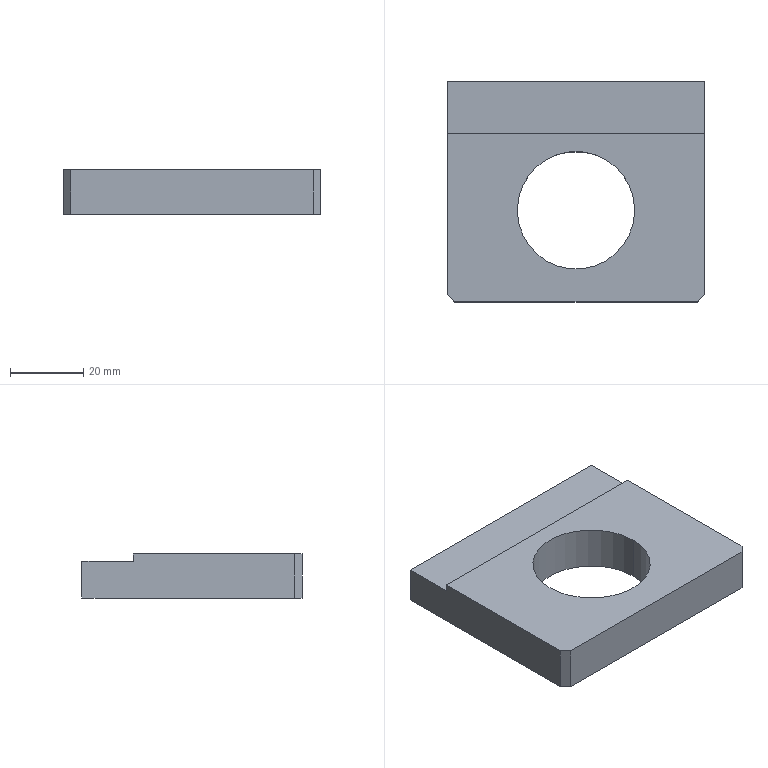Part | STEP file | 2012-06-08-07 | 1 solid | 12 faces | box 70 x 60 x 12 mm | volume 38741 mm3 | plane 10 | cylinder 2 | commonest cylinder face diameters 32 x2
STEP:
#1=CARTESIAN_POINT('',(0.,0.,0.));
#2=DIRECTION('',(0.,0.,1.));
#3=DIRECTION('',(1.,0.,0.));
#4=AXIS2_PLACEMENT_3D('',#1,#2,#3);
#5=CARTESIAN_POINT('',(-16.,-5.,12.));
#6=VERTEX_POINT('',#5);
#7=CARTESIAN_POINT('',(-16.,-5.,0.));
#8=VERTEX_POINT('',#7);
#9=CARTESIAN_POINT('',(-16.,-5.,12.));
#10=DIRECTION('',(0.,0.,-1.));
#11=VECTOR('',#10,1.);
#12=LINE('',#9,#11);
#13=CARTESIAN_POINT('',(0.,-5.,12.));
#14=DIRECTION('',(0.,0.,-1.));
#15=DIRECTION('',(-1.,0.,0.));
#16=AXIS2_PLACEMENT_3D('',#13,#14,#15);
#17=CYLINDRICAL_SURFACE('',#16,16.);
#18=CARTESIAN_POINT('',(6.283,0.));
#19=DIRECTION('',(0.,1.));
#20=VECTOR('',#19,1.);
#21=LINE('',#18,#20);
#22=(GEOMETRIC_REPRESENTATION_CONTEXT(2)PARAMETRIC_REPRESENTATION_CONTEXT()REPRESENTATION_CONTEXT('',''));
#23=DEFINITIONAL_REPRESENTATION('',(#21),#22);
#24=PCURVE('',#17,#23);
#25=CARTESIAN_POINT('',(0.,-5.,12.));
#26=DIRECTION('',(0.,0.,-1.));
#27=DIRECTION('',(-1.,0.,0.));
#28=AXIS2_PLACEMENT_3D('',#25,#26,#27);
#29=CYLINDRICAL_SURFACE('',#28,16.);
#30=CARTESIAN_POINT('',(0.,0.));
#31=DIRECTION('',(0.,1.));
#32=VECTOR('',#31,1.);
#33=LINE('',#30,#32);
#34=(GEOMETRIC_REPRESENTATION_CONTEXT(2)PARAMETRIC_REPRESENTATION_CONTEXT()REPRESENTATION_CONTEXT('',''));
#35=DEFINITIONAL_REPRESENTATION('',(#33),#34);
#36=PCURVE('',#29,#35);
#37=SURFACE_CURVE('',#12,(#24,#36),.PCURVE_S1.);
#38=EDGE_CURVE('',#6,#8,#37,.T.);
#39=ORIENTED_EDGE('',*,*,#38,.T.);
#40=CARTESIAN_POINT('',(16.,-5.,0.));
#41=VERTEX_POINT('',#40);
#42=CARTESIAN_POINT('',(0.,-5.,0.));
#43=DIRECTION('',(0.,0.,1.));
#44=DIRECTION('',(1.,0.,0.));
#45=AXIS2_PLACEMENT_3D('',#42,#43,#44);
#46=CIRCLE('',#45,16.);
#47=CARTESIAN_POINT('',(9.425,12.));
#48=DIRECTION('',(-1.,0.));
#49=VECTOR('',#48,1.);
#50=LINE('',#47,#49);
#51=(GEOMETRIC_REPRESENTATION_CONTEXT(2)PARAMETRIC_REPRESENTATION_CONTEXT()REPRESENTATION_CONTEXT('',''));
#52=DEFINITIONAL_REPRESENTATION('',(#50),#51);
#53=PCURVE('',#17,#52);
#54=CARTESIAN_POINT('',(35.,-30.,0.));
#55=DIRECTION('',(0.,0.,1.));
#56=DIRECTION('',(1.,0.,0.));
#57=AXIS2_PLACEMENT_3D('',#54,#55,#56);
#58=PLANE('',#57);
#59=CARTESIAN_POINT('',(-35.,25.));
#60=DIRECTION('',(1.,0.));
#61=AXIS2_PLACEMENT_2D('',#59,#60);
#62=CIRCLE('',#61,16.);
#63=(GEOMETRIC_REPRESENTATION_CONTEXT(2)PARAMETRIC_REPRESENTATION_CONTEXT()REPRESENTATION_CONTEXT('',''));
#64=DEFINITIONAL_REPRESENTATION('',(#62),#63);
#65=PCURVE('',#58,#64);
#66=SURFACE_CURVE('',#46,(#53,#65),.PCURVE_S1.);
#67=EDGE_CURVE('',#8,#41,#66,.T.);
#68=ORIENTED_EDGE('',*,*,#67,.T.);
#69=CARTESIAN_POINT('',(16.,-5.,12.));
#70=VERTEX_POINT('',#69);
#71=CARTESIAN_POINT('',(16.,-5.,12.));
#72=DIRECTION('',(0.,0.,-1.));
#73=VECTOR('',#72,1.);
#74=LINE('',#71,#73);
#75=CARTESIAN_POINT('',(3.142,0.));
#76=DIRECTION('',(0.,1.));
#77=VECTOR('',#76,1.);
#78=LINE('',#75,#77);
#79=(GEOMETRIC_REPRESENTATION_CONTEXT(2)PARAMETRIC_REPRESENTATION_CONTEXT()REPRESENTATION_CONTEXT('',''));
#80=DEFINITIONAL_REPRESENTATION('',(#78),#79);
#81=PCURVE('',#17,#80);
#82=CARTESIAN_POINT('',(3.142,0.));
#83=DIRECTION('',(0.,1.));
#84=VECTOR('',#83,1.);
#85=LINE('',#82,#84);
#86=(GEOMETRIC_REPRESENTATION_CONTEXT(2)PARAMETRIC_REPRESENTATION_CONTEXT()REPRESENTATION_CONTEXT('',''));
#87=DEFINITIONAL_REPRESENTATION('',(#85),#86);
#88=PCURVE('',#29,#87);
#89=SURFACE_CURVE('',#74,(#81,#88),.PCURVE_S1.);
#90=EDGE_CURVE('',#70,#41,#89,.T.);
#91=ORIENTED_EDGE('',*,*,#90,.F.);
#92=CARTESIAN_POINT('',(0.,-5.,12.));
#93=DIRECTION('',(0.,0.,1.));
#94=DIRECTION('',(1.,0.,0.));
#95=AXIS2_PLACEMENT_3D('',#92,#93,#94);
#96=CIRCLE('',#95,16.);
#97=CARTESIAN_POINT('',(9.425,0.));
#98=DIRECTION('',(-1.,0.));
#99=VECTOR('',#98,1.);
#100=LINE('',#97,#99);
#101=(GEOMETRIC_REPRESENTATION_CONTEXT(2)PARAMETRIC_REPRESENTATION_CONTEXT()REPRESENTATION_CONTEXT('',''));
#102=DEFINITIONAL_REPRESENTATION('',(#100),#101);
#103=PCURVE('',#17,#102);
#104=CARTESIAN_POINT('',(35.,-30.,12.));
#105=DIRECTION('',(0.,0.,1.));
#106=DIRECTION('',(1.,0.,0.));
#107=AXIS2_PLACEMENT_3D('',#104,#105,#106);
#108=PLANE('',#107);
#109=CARTESIAN_POINT('',(-35.,25.));
#110=DIRECTION('',(1.,0.));
#111=AXIS2_PLACEMENT_2D('',#109,#110);
#112=CIRCLE('',#111,16.);
#113=(GEOMETRIC_REPRESENTATION_CONTEXT(2)PARAMETRIC_REPRESENTATION_CONTEXT()REPRESENTATION_CONTEXT('',''));
#114=DEFINITIONAL_REPRESENTATION('',(#112),#113);
#115=PCURVE('',#108,#114);
#116=SURFACE_CURVE('',#96,(#103,#115),.PCURVE_S1.);
#117=EDGE_CURVE('',#6,#70,#116,.T.);
#118=ORIENTED_EDGE('',*,*,#117,.F.);
#119=EDGE_LOOP('',(#39,#68,#91,#118));
#120=FACE_BOUND('',#119,.F.);
#121=ADVANCED_FACE('',(#120),#17,.F.);
#122=CARTESIAN_POINT('',(35.,30.,10.));
#123=VERTEX_POINT('',#122);
#124=CARTESIAN_POINT('',(-35.,30.,10.));
#125=VERTEX_POINT('',#124);
#126=CARTESIAN_POINT('',(-35.,30.,10.));
#127=DIRECTION('',(-1.,0.,0.));
#128=VECTOR('',#127,1.);
#129=LINE('',#126,#128);
#130=CARTESIAN_POINT('',(-35.,30.,12.));
#131=DIRECTION('',(0.,-1.,0.));
#132=DIRECTION('',(0.,0.,-1.));
#133=AXIS2_PLACEMENT_3D('',#130,#131,#132);
#134=PLANE('',#133);
#135=CARTESIAN_POINT('',(2.,0.));
#136=DIRECTION('',(0.,-1.));
#137=VECTOR('',#136,1.);
#138=LINE('',#135,#137);
#139=(GEOMETRIC_REPRESENTATION_CONTEXT(2)PARAMETRIC_REPRESENTATION_CONTEXT()REPRESENTATION_CONTEXT('',''));
#140=DEFINITIONAL_REPRESENTATION('',(#138),#139);
#141=PCURVE('',#134,#140);
#142=CARTESIAN_POINT('',(-35.,16.,10.));
#143=DIRECTION('',(0.,0.,1.));
#144=DIRECTION('',(1.,0.,0.));
#145=AXIS2_PLACEMENT_3D('',#142,#143,#144);
#146=PLANE('',#145);
#147=CARTESIAN_POINT('',(0.,14.));
#148=DIRECTION('',(-1.,0.));
#149=VECTOR('',#148,1.);
#150=LINE('',#147,#149);
#151=(GEOMETRIC_REPRESENTATION_CONTEXT(2)PARAMETRIC_REPRESENTATION_CONTEXT()REPRESENTATION_CONTEXT('',''));
#152=DEFINITIONAL_REPRESENTATION('',(#150),#151);
#153=PCURVE('',#146,#152);
#154=SURFACE_CURVE('',#129,(#141,#153),.PCURVE_S1.);
#155=EDGE_CURVE('',#123,#125,#154,.T.);
#156=ORIENTED_EDGE('',*,*,#155,.F.);
#157=CARTESIAN_POINT('',(35.,30.,0.));
#158=VERTEX_POINT('',#157);
#159=CARTESIAN_POINT('',(35.,30.,12.));
#160=DIRECTION('',(0.,0.,-1.));
#161=VECTOR('',#160,1.);
#162=LINE('',#159,#161);
#163=CARTESIAN_POINT('',(0.,70.));
#164=DIRECTION('',(1.,0.));
#165=VECTOR('',#164,1.);
#166=LINE('',#163,#165);
#167=(GEOMETRIC_REPRESENTATION_CONTEXT(2)PARAMETRIC_REPRESENTATION_CONTEXT()REPRESENTATION_CONTEXT('',''));
#168=DEFINITIONAL_REPRESENTATION('',(#166),#167);
#169=PCURVE('',#134,#168);
#170=CARTESIAN_POINT('',(35.,30.,12.));
#171=DIRECTION('',(-1.,0.,0.));
#172=DIRECTION('',(0.,0.,1.));
#173=AXIS2_PLACEMENT_3D('',#170,#171,#172);
#174=PLANE('',#173);
#175=CARTESIAN_POINT('',(0.,0.));
#176=DIRECTION('',(-1.,0.));
#177=VECTOR('',#176,1.);
#178=LINE('',#175,#177);
#179=(GEOMETRIC_REPRESENTATION_CONTEXT(2)PARAMETRIC_REPRESENTATION_CONTEXT()REPRESENTATION_CONTEXT('',''));
#180=DEFINITIONAL_REPRESENTATION('',(#178),#179);
#181=PCURVE('',#174,#180);
#182=SURFACE_CURVE('',#162,(#169,#181),.PCURVE_S1.);
#183=EDGE_CURVE('',#123,#158,#182,.T.);
#184=ORIENTED_EDGE('',*,*,#183,.T.);
#185=CARTESIAN_POINT('',(-35.,30.,0.));
#186=VERTEX_POINT('',#185);
#187=CARTESIAN_POINT('',(-35.,30.,0.));
#188=DIRECTION('',(-1.,0.,0.));
#189=VECTOR('',#188,1.);
#190=LINE('',#187,#189);
#191=CARTESIAN_POINT('',(12.,0.));
#192=DIRECTION('',(0.,-1.));
#193=VECTOR('',#192,1.);
#194=LINE('',#191,#193);
#195=(GEOMETRIC_REPRESENTATION_CONTEXT(2)PARAMETRIC_REPRESENTATION_CONTEXT()REPRESENTATION_CONTEXT('',''));
#196=DEFINITIONAL_REPRESENTATION('',(#194),#195);
#197=PCURVE('',#134,#196);
#198=CARTESIAN_POINT('',(-70.,60.));
#199=DIRECTION('',(-1.,0.));
#200=VECTOR('',#199,1.);
#201=LINE('',#198,#200);
#202=(GEOMETRIC_REPRESENTATION_CONTEXT(2)PARAMETRIC_REPRESENTATION_CONTEXT()REPRESENTATION_CONTEXT('',''));
#203=DEFINITIONAL_REPRESENTATION('',(#201),#202);
#204=PCURVE('',#58,#203);
#205=SURFACE_CURVE('',#190,(#197,#204),.PCURVE_S1.);
#206=EDGE_CURVE('',#158,#186,#205,.T.);
#207=ORIENTED_EDGE('',*,*,#206,.T.);
#208=CARTESIAN_POINT('',(-35.,30.,12.));
#209=DIRECTION('',(0.,0.,-1.));
#210=VECTOR('',#209,1.);
#211=LINE('',#208,#210);
#212=CARTESIAN_POINT('',(0.,0.));
#213=DIRECTION('',(1.,0.));
#214=VECTOR('',#213,1.);
#215=LINE('',#212,#214);
#216=(GEOMETRIC_REPRESENTATION_CONTEXT(2)PARAMETRIC_REPRESENTATION_CONTEXT()REPRESENTATION_CONTEXT('',''));
#217=DEFINITIONAL_REPRESENTATION('',(#215),#216);
#218=PCURVE('',#134,#217);
#219=CARTESIAN_POINT('',(-35.,30.,12.));
#220=DIRECTION('',(1.,0.,0.));
#221=DIRECTION('',(0.,1.,0.));
#222=AXIS2_PLACEMENT_3D('',#219,#220,#221);
#223=PLANE('',#222);
#224=CARTESIAN_POINT('',(0.,0.));
#225=DIRECTION('',(0.,-1.));
#226=VECTOR('',#225,1.);
#227=LINE('',#224,#226);
#228=(GEOMETRIC_REPRESENTATION_CONTEXT(2)PARAMETRIC_REPRESENTATION_CONTEXT()REPRESENTATION_CONTEXT('',''));
#229=DEFINITIONAL_REPRESENTATION('',(#227),#228);
#230=PCURVE('',#223,#229);
#231=SURFACE_CURVE('',#211,(#218,#230),.PCURVE_S1.);
#232=EDGE_CURVE('',#125,#186,#231,.T.);
#233=ORIENTED_EDGE('',*,*,#232,.F.);
#234=EDGE_LOOP('',(#156,#184,#207,#233));
#235=FACE_BOUND('',#234,.T.);
#236=ADVANCED_FACE('',(#235),#134,.F.);
#237=CARTESIAN_POINT('',(-33.,-30.,12.));
#238=VERTEX_POINT('',#237);
#239=CARTESIAN_POINT('',(33.,-30.,12.));
#240=VERTEX_POINT('',#239);
#241=CARTESIAN_POINT('',(-35.,-30.,12.));
#242=DIRECTION('',(1.,0.,0.));
#243=VECTOR('',#242,1.);
#244=LINE('',#241,#243);
#245=CARTESIAN_POINT('',(-70.,0.));
#246=DIRECTION('',(1.,0.));
#247=VECTOR('',#246,1.);
#248=LINE('',#245,#247);
#249=(GEOMETRIC_REPRESENTATION_CONTEXT(2)PARAMETRIC_REPRESENTATION_CONTEXT()REPRESENTATION_CONTEXT('',''));
#250=DEFINITIONAL_REPRESENTATION('',(#248),#249);
#251=PCURVE('',#108,#250);
#252=CARTESIAN_POINT('',(-35.,-30.,12.));
#253=DIRECTION('',(0.,1.,0.));
#254=DIRECTION('',(0.,0.,1.));
#255=AXIS2_PLACEMENT_3D('',#252,#253,#254);
#256=PLANE('',#255);
#257=CARTESIAN_POINT('',(0.,0.));
#258=DIRECTION('',(0.,1.));
#259=VECTOR('',#258,1.);
#260=LINE('',#257,#259);
#261=(GEOMETRIC_REPRESENTATION_CONTEXT(2)PARAMETRIC_REPRESENTATION_CONTEXT()REPRESENTATION_CONTEXT('',''));
#262=DEFINITIONAL_REPRESENTATION('',(#260),#261);
#263=PCURVE('',#256,#262);
#264=SURFACE_CURVE('',#244,(#251,#263),.PCURVE_S1.);
#265=EDGE_CURVE('',#238,#240,#264,.T.);
#266=ORIENTED_EDGE('',*,*,#265,.T.);
#267=CARTESIAN_POINT('',(35.,-28.,12.));
#268=VERTEX_POINT('',#267);
#269=CARTESIAN_POINT('',(34.,-29.,12.));
#270=DIRECTION('',(0.7071,0.7071,0.));
#271=VECTOR('',#270,1.);
#272=LINE('',#269,#271);
#273=CARTESIAN_POINT('',(-1.,1.));
#274=DIRECTION('',(0.7071,0.7071));
#275=VECTOR('',#274,1.);
#276=LINE('',#273,#275);
#277=(GEOMETRIC_REPRESENTATION_CONTEXT(2)PARAMETRIC_REPRESENTATION_CONTEXT()REPRESENTATION_CONTEXT('',''));
#278=DEFINITIONAL_REPRESENTATION('',(#276),#277);
#279=PCURVE('',#108,#278);
#280=CARTESIAN_POINT('',(35.,-28.,12.));
#281=DIRECTION('',(-0.7071,0.7071,0.));
#282=DIRECTION('',(-0.7071,-0.7071,0.));
#283=AXIS2_PLACEMENT_3D('',#280,#281,#282);
#284=PLANE('',#283);
#285=CARTESIAN_POINT('',(1.414,0.));
#286=DIRECTION('',(-1.,0.));
#287=VECTOR('',#286,1.);
#288=LINE('',#285,#287);
#289=(GEOMETRIC_REPRESENTATION_CONTEXT(2)PARAMETRIC_REPRESENTATION_CONTEXT()REPRESENTATION_CONTEXT('',''));
#290=DEFINITIONAL_REPRESENTATION('',(#288),#289);
#291=PCURVE('',#284,#290);
#292=SURFACE_CURVE('',#272,(#279,#291),.PCURVE_S1.);
#293=EDGE_CURVE('',#240,#268,#292,.T.);
#294=ORIENTED_EDGE('',*,*,#293,.T.);
#295=CARTESIAN_POINT('',(35.,16.,12.));
#296=VERTEX_POINT('',#295);
#297=CARTESIAN_POINT('',(35.,30.,12.));
#298=DIRECTION('',(0.,1.,0.));
#299=VECTOR('',#298,1.);
#300=LINE('',#297,#299);
#301=CARTESIAN_POINT('',(0.,60.));
#302=DIRECTION('',(0.,1.));
#303=VECTOR('',#302,1.);
#304=LINE('',#301,#303);
#305=(GEOMETRIC_REPRESENTATION_CONTEXT(2)PARAMETRIC_REPRESENTATION_CONTEXT()REPRESENTATION_CONTEXT('',''));
#306=DEFINITIONAL_REPRESENTATION('',(#304),#305);
#307=PCURVE('',#108,#306);
#308=CARTESIAN_POINT('',(0.,0.));
#309=DIRECTION('',(0.,1.));
#310=VECTOR('',#309,1.);
#311=LINE('',#308,#310);
#312=(GEOMETRIC_REPRESENTATION_CONTEXT(2)PARAMETRIC_REPRESENTATION_CONTEXT()REPRESENTATION_CONTEXT('',''));
#313=DEFINITIONAL_REPRESENTATION('',(#311),#312);
#314=PCURVE('',#174,#313);
#315=SURFACE_CURVE('',#300,(#307,#314),.PCURVE_S1.);
#316=EDGE_CURVE('',#268,#296,#315,.T.);
#317=ORIENTED_EDGE('',*,*,#316,.T.);
#318=CARTESIAN_POINT('',(-35.,16.,12.));
#319=VERTEX_POINT('',#318);
#320=CARTESIAN_POINT('',(-35.,16.,12.));
#321=DIRECTION('',(1.,0.,0.));
#322=VECTOR('',#321,1.);
#323=LINE('',#320,#322);
#324=CARTESIAN_POINT('',(-70.,46.));
#325=DIRECTION('',(1.,0.));
#326=VECTOR('',#325,1.);
#327=LINE('',#324,#326);
#328=(GEOMETRIC_REPRESENTATION_CONTEXT(2)PARAMETRIC_REPRESENTATION_CONTEXT()REPRESENTATION_CONTEXT('',''));
#329=DEFINITIONAL_REPRESENTATION('',(#327),#328);
#330=PCURVE('',#108,#329);
#331=CARTESIAN_POINT('',(-35.,16.,10.));
#332=DIRECTION('',(0.,-1.,0.));
#333=DIRECTION('',(0.,0.,-1.));
#334=AXIS2_PLACEMENT_3D('',#331,#332,#333);
#335=PLANE('',#334);
#336=CARTESIAN_POINT('',(-2.,0.));
#337=DIRECTION('',(0.,1.));
#338=VECTOR('',#337,1.);
#339=LINE('',#336,#338);
#340=(GEOMETRIC_REPRESENTATION_CONTEXT(2)PARAMETRIC_REPRESENTATION_CONTEXT()REPRESENTATION_CONTEXT('',''));
#341=DEFINITIONAL_REPRESENTATION('',(#339),#340);
#342=PCURVE('',#335,#341);
#343=SURFACE_CURVE('',#323,(#330,#342),.PCURVE_S1.);
#344=EDGE_CURVE('',#319,#296,#343,.T.);
#345=ORIENTED_EDGE('',*,*,#344,.F.);
#346=CARTESIAN_POINT('',(-35.,-28.,12.));
#347=VERTEX_POINT('',#346);
#348=CARTESIAN_POINT('',(-35.,30.,12.));
#349=DIRECTION('',(0.,-1.,0.));
#350=VECTOR('',#349,1.);
#351=LINE('',#348,#350);
#352=CARTESIAN_POINT('',(-70.,60.));
#353=DIRECTION('',(0.,-1.));
#354=VECTOR('',#353,1.);
#355=LINE('',#352,#354);
#356=(GEOMETRIC_REPRESENTATION_CONTEXT(2)PARAMETRIC_REPRESENTATION_CONTEXT()REPRESENTATION_CONTEXT('',''));
#357=DEFINITIONAL_REPRESENTATION('',(#355),#356);
#358=PCURVE('',#108,#357);
#359=CARTESIAN_POINT('',(0.,0.));
#360=DIRECTION('',(-1.,0.));
#361=VECTOR('',#360,1.);
#362=LINE('',#359,#361);
#363=(GEOMETRIC_REPRESENTATION_CONTEXT(2)PARAMETRIC_REPRESENTATION_CONTEXT()REPRESENTATION_CONTEXT('',''));
#364=DEFINITIONAL_REPRESENTATION('',(#362),#363);
#365=PCURVE('',#223,#364);
#366=SURFACE_CURVE('',#351,(#358,#365),.PCURVE_S1.);
#367=EDGE_CURVE('',#319,#347,#366,.T.);
#368=ORIENTED_EDGE('',*,*,#367,.T.);
#369=CARTESIAN_POINT('',(1.,-64.,12.));
#370=DIRECTION('',(0.7071,-0.7071,0.));
#371=VECTOR('',#370,1.);
#372=LINE('',#369,#371);
#373=CARTESIAN_POINT('',(-34.,-34.));
#374=DIRECTION('',(0.7071,-0.7071));
#375=VECTOR('',#374,1.);
#376=LINE('',#373,#375);
#377=(GEOMETRIC_REPRESENTATION_CONTEXT(2)PARAMETRIC_REPRESENTATION_CONTEXT()REPRESENTATION_CONTEXT('',''));
#378=DEFINITIONAL_REPRESENTATION('',(#376),#377);
#379=PCURVE('',#108,#378);
#380=CARTESIAN_POINT('',(-33.,-30.,12.));
#381=DIRECTION('',(0.7071,0.7071,0.));
#382=DIRECTION('',(-0.7071,0.7071,0.));
#383=AXIS2_PLACEMENT_3D('',#380,#381,#382);
#384=PLANE('',#383);
#385=CARTESIAN_POINT('',(-48.083,0.));
#386=DIRECTION('',(-1.,0.));
#387=VECTOR('',#386,1.);
#388=LINE('',#385,#387);
#389=(GEOMETRIC_REPRESENTATION_CONTEXT(2)PARAMETRIC_REPRESENTATION_CONTEXT()REPRESENTATION_CONTEXT('',''));
#390=DEFINITIONAL_REPRESENTATION('',(#388),#389);
#391=PCURVE('',#384,#390);
#392=SURFACE_CURVE('',#372,(#379,#391),.PCURVE_S1.);
#393=EDGE_CURVE('',#347,#238,#392,.T.);
#394=ORIENTED_EDGE('',*,*,#393,.T.);
#395=EDGE_LOOP('',(#266,#294,#317,#345,#368,#394));
#396=FACE_BOUND('',#395,.T.);
#397=ORIENTED_EDGE('',*,*,#117,.F.);
#398=CARTESIAN_POINT('',(0.,-5.,12.));
#399=DIRECTION('',(0.,0.,1.));
#400=DIRECTION('',(1.,0.,0.));
#401=AXIS2_PLACEMENT_3D('',#398,#399,#400);
#402=CIRCLE('',#401,16.);
#403=CARTESIAN_POINT('',(-35.,25.));
#404=DIRECTION('',(1.,0.));
#405=AXIS2_PLACEMENT_2D('',#403,#404);
#406=CIRCLE('',#405,16.);
#407=(GEOMETRIC_REPRESENTATION_CONTEXT(2)PARAMETRIC_REPRESENTATION_CONTEXT()REPRESENTATION_CONTEXT('',''));
#408=DEFINITIONAL_REPRESENTATION('',(#406),#407);
#409=PCURVE('',#108,#408);
#410=CARTESIAN_POINT('',(3.142,0.));
#411=DIRECTION('',(-1.,0.));
#412=VECTOR('',#411,1.);
#413=LINE('',#410,#412);
#414=(GEOMETRIC_REPRESENTATION_CONTEXT(2)PARAMETRIC_REPRESENTATION_CONTEXT()REPRESENTATION_CONTEXT('',''));
#415=DEFINITIONAL_REPRESENTATION('',(#413),#414);
#416=PCURVE('',#29,#415);
#417=SURFACE_CURVE('',#402,(#409,#416),.PCURVE_S1.);
#418=EDGE_CURVE('',#70,#6,#417,.T.);
#419=ORIENTED_EDGE('',*,*,#418,.F.);
#420=EDGE_LOOP('',(#397,#419));
#421=FACE_BOUND('',#420,.T.);
#422=ADVANCED_FACE('',(#396,#421),#108,.T.);
#423=CARTESIAN_POINT('',(35.,-28.,0.));
#424=VERTEX_POINT('',#423);
#425=CARTESIAN_POINT('',(35.,30.,0.));
#426=DIRECTION('',(0.,1.,0.));
#427=VECTOR('',#426,1.);
#428=LINE('',#425,#427);
#429=CARTESIAN_POINT('',(0.,60.));
#430=DIRECTION('',(0.,1.));
#431=VECTOR('',#430,1.);
#432=LINE('',#429,#431);
#433=(GEOMETRIC_REPRESENTATION_CONTEXT(2)PARAMETRIC_REPRESENTATION_CONTEXT()REPRESENTATION_CONTEXT('',''));
#434=DEFINITIONAL_REPRESENTATION('',(#432),#433);
#435=PCURVE('',#58,#434);
#436=CARTESIAN_POINT('',(-12.,0.));
#437=DIRECTION('',(0.,1.));
#438=VECTOR('',#437,1.);
#439=LINE('',#436,#438);
#440=(GEOMETRIC_REPRESENTATION_CONTEXT(2)PARAMETRIC_REPRESENTATION_CONTEXT()REPRESENTATION_CONTEXT('',''));
#441=DEFINITIONAL_REPRESENTATION('',(#439),#440);
#442=PCURVE('',#174,#441);
#443=SURFACE_CURVE('',#428,(#435,#442),.PCURVE_S1.);
#444=EDGE_CURVE('',#424,#158,#443,.T.);
#445=ORIENTED_EDGE('',*,*,#444,.F.);
#446=CARTESIAN_POINT('',(33.,-30.,0.));
#447=VERTEX_POINT('',#446);
#448=CARTESIAN_POINT('',(35.,-28.,0.));
#449=DIRECTION('',(-0.7071,-0.7071,0.));
#450=VECTOR('',#449,1.);
#451=LINE('',#448,#450);
#452=CARTESIAN_POINT('',(0.,2.));
#453=DIRECTION('',(-0.7071,-0.7071));
#454=VECTOR('',#453,1.);
#455=LINE('',#452,#454);
#456=(GEOMETRIC_REPRESENTATION_CONTEXT(2)PARAMETRIC_REPRESENTATION_CONTEXT()REPRESENTATION_CONTEXT('',''));
#457=DEFINITIONAL_REPRESENTATION('',(#455),#456);
#458=PCURVE('',#58,#457);
#459=CARTESIAN_POINT('',(0.,-12.));
#460=DIRECTION('',(1.,0.));
#461=VECTOR('',#460,1.);
#462=LINE('',#459,#461);
#463=(GEOMETRIC_REPRESENTATION_CONTEXT(2)PARAMETRIC_REPRESENTATION_CONTEXT()REPRESENTATION_CONTEXT('',''));
#464=DEFINITIONAL_REPRESENTATION('',(#462),#463);
#465=PCURVE('',#284,#464);
#466=SURFACE_CURVE('',#451,(#458,#465),.PCURVE_S1.);
#467=EDGE_CURVE('',#424,#447,#466,.T.);
#468=ORIENTED_EDGE('',*,*,#467,.T.);
#469=CARTESIAN_POINT('',(-33.,-30.,0.));
#470=VERTEX_POINT('',#469);
#471=CARTESIAN_POINT('',(-35.,-30.,0.));
#472=DIRECTION('',(1.,0.,0.));
#473=VECTOR('',#472,1.);
#474=LINE('',#471,#473);
#475=CARTESIAN_POINT('',(-70.,0.));
#476=DIRECTION('',(1.,0.));
#477=VECTOR('',#476,1.);
#478=LINE('',#475,#477);
#479=(GEOMETRIC_REPRESENTATION_CONTEXT(2)PARAMETRIC_REPRESENTATION_CONTEXT()REPRESENTATION_CONTEXT('',''));
#480=DEFINITIONAL_REPRESENTATION('',(#478),#479);
#481=PCURVE('',#58,#480);
#482=CARTESIAN_POINT('',(-12.,0.));
#483=DIRECTION('',(0.,1.));
#484=VECTOR('',#483,1.);
#485=LINE('',#482,#484);
#486=(GEOMETRIC_REPRESENTATION_CONTEXT(2)PARAMETRIC_REPRESENTATION_CONTEXT()REPRESENTATION_CONTEXT('',''));
#487=DEFINITIONAL_REPRESENTATION('',(#485),#486);
#488=PCURVE('',#256,#487);
#489=SURFACE_CURVE('',#474,(#481,#488),.PCURVE_S1.);
#490=EDGE_CURVE('',#470,#447,#489,.T.);
#491=ORIENTED_EDGE('',*,*,#490,.F.);
#492=CARTESIAN_POINT('',(-35.,-28.,0.));
#493=VERTEX_POINT('',#492);
#494=CARTESIAN_POINT('',(-33.,-30.,0.));
#495=DIRECTION('',(-0.7071,0.7071,0.));
#496=VECTOR('',#495,1.);
#497=LINE('',#494,#496);
#498=CARTESIAN_POINT('',(-68.,0.));
#499=DIRECTION('',(-0.7071,0.7071));
#500=VECTOR('',#499,1.);
#501=LINE('',#498,#500);
#502=(GEOMETRIC_REPRESENTATION_CONTEXT(2)PARAMETRIC_REPRESENTATION_CONTEXT()REPRESENTATION_CONTEXT('',''));
#503=DEFINITIONAL_REPRESENTATION('',(#501),#502);
#504=PCURVE('',#58,#503);
#505=CARTESIAN_POINT('',(0.,-12.));
#506=DIRECTION('',(1.,0.));
#507=VECTOR('',#506,1.);
#508=LINE('',#505,#507);
#509=(GEOMETRIC_REPRESENTATION_CONTEXT(2)PARAMETRIC_REPRESENTATION_CONTEXT()REPRESENTATION_CONTEXT('',''));
#510=DEFINITIONAL_REPRESENTATION('',(#508),#509);
#511=PCURVE('',#384,#510);
#512=SURFACE_CURVE('',#497,(#504,#511),.PCURVE_S1.);
#513=EDGE_CURVE('',#470,#493,#512,.T.);
#514=ORIENTED_EDGE('',*,*,#513,.T.);
#515=CARTESIAN_POINT('',(-35.,30.,0.));
#516=DIRECTION('',(0.,-1.,0.));
#517=VECTOR('',#516,1.);
#518=LINE('',#515,#517);
#519=CARTESIAN_POINT('',(-70.,60.));
#520=DIRECTION('',(0.,-1.));
#521=VECTOR('',#520,1.);
#522=LINE('',#519,#521);
#523=(GEOMETRIC_REPRESENTATION_CONTEXT(2)PARAMETRIC_REPRESENTATION_CONTEXT()REPRESENTATION_CONTEXT('',''));
#524=DEFINITIONAL_REPRESENTATION('',(#522),#523);
#525=PCURVE('',#58,#524);
#526=CARTESIAN_POINT('',(0.,-12.));
#527=DIRECTION('',(-1.,0.));
#528=VECTOR('',#527,1.);
#529=LINE('',#526,#528);
#530=(GEOMETRIC_REPRESENTATION_CONTEXT(2)PARAMETRIC_REPRESENTATION_CONTEXT()REPRESENTATION_CONTEXT('',''));
#531=DEFINITIONAL_REPRESENTATION('',(#529),#530);
#532=PCURVE('',#223,#531);
#533=SURFACE_CURVE('',#518,(#525,#532),.PCURVE_S1.);
#534=EDGE_CURVE('',#186,#493,#533,.T.);
#535=ORIENTED_EDGE('',*,*,#534,.F.);
#536=ORIENTED_EDGE('',*,*,#206,.F.);
#537=EDGE_LOOP('',(#445,#468,#491,#514,#535,#536));
#538=FACE_BOUND('',#537,.T.);
#539=ORIENTED_EDGE('',*,*,#67,.T.);
#540=CARTESIAN_POINT('',(0.,-5.,0.));
#541=DIRECTION('',(0.,0.,1.));
#542=DIRECTION('',(1.,0.,0.));
#543=AXIS2_PLACEMENT_3D('',#540,#541,#542);
#544=CIRCLE('',#543,16.);
#545=CARTESIAN_POINT('',(-35.,25.));
#546=DIRECTION('',(1.,0.));
#547=AXIS2_PLACEMENT_2D('',#545,#546);
#548=CIRCLE('',#547,16.);
#549=(GEOMETRIC_REPRESENTATION_CONTEXT(2)PARAMETRIC_REPRESENTATION_CONTEXT()REPRESENTATION_CONTEXT('',''));
#550=DEFINITIONAL_REPRESENTATION('',(#548),#549);
#551=PCURVE('',#58,#550);
#552=CARTESIAN_POINT('',(3.142,12.));
#553=DIRECTION('',(-1.,0.));
#554=VECTOR('',#553,1.);
#555=LINE('',#552,#554);
#556=(GEOMETRIC_REPRESENTATION_CONTEXT(2)PARAMETRIC_REPRESENTATION_CONTEXT()REPRESENTATION_CONTEXT('',''));
#557=DEFINITIONAL_REPRESENTATION('',(#555),#556);
#558=PCURVE('',#29,#557);
#559=SURFACE_CURVE('',#544,(#551,#558),.PCURVE_S1.);
#560=EDGE_CURVE('',#41,#8,#559,.T.);
#561=ORIENTED_EDGE('',*,*,#560,.T.);
#562=EDGE_LOOP('',(#539,#561));
#563=FACE_BOUND('',#562,.T.);
#564=ADVANCED_FACE('',(#538,#563),#58,.F.);
#565=ORIENTED_EDGE('',*,*,#316,.F.);
#566=CARTESIAN_POINT('',(35.,-28.,12.));
#567=DIRECTION('',(0.,0.,-1.));
#568=VECTOR('',#567,1.);
#569=LINE('',#566,#568);
#570=CARTESIAN_POINT('',(0.,-58.));
#571=DIRECTION('',(-1.,0.));
#572=VECTOR('',#571,1.);
#573=LINE('',#570,#572);
#574=(GEOMETRIC_REPRESENTATION_CONTEXT(2)PARAMETRIC_REPRESENTATION_CONTEXT()REPRESENTATION_CONTEXT('',''));
#575=DEFINITIONAL_REPRESENTATION('',(#573),#574);
#576=PCURVE('',#174,#575);
#577=CARTESIAN_POINT('',(0.,0.));
#578=DIRECTION('',(0.,-1.));
#579=VECTOR('',#578,1.);
#580=LINE('',#577,#579);
#581=(GEOMETRIC_REPRESENTATION_CONTEXT(2)PARAMETRIC_REPRESENTATION_CONTEXT()REPRESENTATION_CONTEXT('',''));
#582=DEFINITIONAL_REPRESENTATION('',(#580),#581);
#583=PCURVE('',#284,#582);
#584=SURFACE_CURVE('',#569,(#576,#583),.PCURVE_S1.);
#585=EDGE_CURVE('',#268,#424,#584,.T.);
#586=ORIENTED_EDGE('',*,*,#585,.T.);
#587=ORIENTED_EDGE('',*,*,#444,.T.);
#588=ORIENTED_EDGE('',*,*,#183,.F.);
#589=CARTESIAN_POINT('',(35.,16.,10.));
#590=VERTEX_POINT('',#589);
#591=CARTESIAN_POINT('',(35.,30.,10.));
#592=DIRECTION('',(0.,1.,0.));
#593=VECTOR('',#592,1.);
#594=LINE('',#591,#593);
#595=CARTESIAN_POINT('',(-2.,0.));
#596=DIRECTION('',(0.,1.));
#597=VECTOR('',#596,1.);
#598=LINE('',#595,#597);
#599=(GEOMETRIC_REPRESENTATION_CONTEXT(2)PARAMETRIC_REPRESENTATION_CONTEXT()REPRESENTATION_CONTEXT('',''));
#600=DEFINITIONAL_REPRESENTATION('',(#598),#599);
#601=PCURVE('',#174,#600);
#602=CARTESIAN_POINT('',(70.,14.));
#603=DIRECTION('',(0.,1.));
#604=VECTOR('',#603,1.);
#605=LINE('',#602,#604);
#606=(GEOMETRIC_REPRESENTATION_CONTEXT(2)PARAMETRIC_REPRESENTATION_CONTEXT()REPRESENTATION_CONTEXT('',''));
#607=DEFINITIONAL_REPRESENTATION('',(#605),#606);
#608=PCURVE('',#146,#607);
#609=SURFACE_CURVE('',#594,(#601,#608),.PCURVE_S1.);
#610=EDGE_CURVE('',#590,#123,#609,.T.);
#611=ORIENTED_EDGE('',*,*,#610,.F.);
#612=CARTESIAN_POINT('',(35.,16.,10.));
#613=DIRECTION('',(0.,0.,1.));
#614=VECTOR('',#613,1.);
#615=LINE('',#612,#614);
#616=CARTESIAN_POINT('',(-2.,-14.));
#617=DIRECTION('',(1.,0.));
#618=VECTOR('',#617,1.);
#619=LINE('',#616,#618);
#620=(GEOMETRIC_REPRESENTATION_CONTEXT(2)PARAMETRIC_REPRESENTATION_CONTEXT()REPRESENTATION_CONTEXT('',''));
#621=DEFINITIONAL_REPRESENTATION('',(#619),#620);
#622=PCURVE('',#174,#621);
#623=CARTESIAN_POINT('',(0.,70.));
#624=DIRECTION('',(-1.,0.));
#625=VECTOR('',#624,1.);
#626=LINE('',#623,#625);
#627=(GEOMETRIC_REPRESENTATION_CONTEXT(2)PARAMETRIC_REPRESENTATION_CONTEXT()REPRESENTATION_CONTEXT('',''));
#628=DEFINITIONAL_REPRESENTATION('',(#626),#627);
#629=PCURVE('',#335,#628);
#630=SURFACE_CURVE('',#615,(#622,#629),.PCURVE_S1.);
#631=EDGE_CURVE('',#590,#296,#630,.T.);
#632=ORIENTED_EDGE('',*,*,#631,.T.);
#633=EDGE_LOOP('',(#565,#586,#587,#588,#611,#632));
#634=FACE_BOUND('',#633,.T.);
#635=ADVANCED_FACE('',(#634),#174,.F.);
#636=ORIENTED_EDGE('',*,*,#534,.T.);
#637=CARTESIAN_POINT('',(-35.,-28.,12.));
#638=DIRECTION('',(0.,0.,1.));
#639=VECTOR('',#638,1.);
#640=LINE('',#637,#639);
#641=CARTESIAN_POINT('',(-58.,0.));
#642=DIRECTION('',(0.,1.));
#643=VECTOR('',#642,1.);
#644=LINE('',#641,#643);
#645=(GEOMETRIC_REPRESENTATION_CONTEXT(2)PARAMETRIC_REPRESENTATION_CONTEXT()REPRESENTATION_CONTEXT('',''));
#646=DEFINITIONAL_REPRESENTATION('',(#644),#645);
#647=PCURVE('',#223,#646);
#648=CARTESIAN_POINT('',(2.828,0.));
#649=DIRECTION('',(0.,1.));
#650=VECTOR('',#649,1.);
#651=LINE('',#648,#650);
#652=(GEOMETRIC_REPRESENTATION_CONTEXT(2)PARAMETRIC_REPRESENTATION_CONTEXT()REPRESENTATION_CONTEXT('',''));
#653=DEFINITIONAL_REPRESENTATION('',(#651),#652);
#654=PCURVE('',#384,#653);
#655=SURFACE_CURVE('',#640,(#647,#654),.PCURVE_S1.);
#656=EDGE_CURVE('',#493,#347,#655,.T.);
#657=ORIENTED_EDGE('',*,*,#656,.T.);
#658=ORIENTED_EDGE('',*,*,#367,.F.);
#659=CARTESIAN_POINT('',(-35.,16.,10.));
#660=VERTEX_POINT('',#659);
#661=CARTESIAN_POINT('',(-35.,16.,10.));
#662=DIRECTION('',(0.,0.,1.));
#663=VECTOR('',#662,1.);
#664=LINE('',#661,#663);
#665=CARTESIAN_POINT('',(-14.,-2.));
#666=DIRECTION('',(0.,1.));
#667=VECTOR('',#666,1.);
#668=LINE('',#665,#667);
#669=(GEOMETRIC_REPRESENTATION_CONTEXT(2)PARAMETRIC_REPRESENTATION_CONTEXT()REPRESENTATION_CONTEXT('',''));
#670=DEFINITIONAL_REPRESENTATION('',(#668),#669);
#671=PCURVE('',#223,#670);
#672=CARTESIAN_POINT('',(0.,0.));
#673=DIRECTION('',(-1.,0.));
#674=VECTOR('',#673,1.);
#675=LINE('',#672,#674);
#676=(GEOMETRIC_REPRESENTATION_CONTEXT(2)PARAMETRIC_REPRESENTATION_CONTEXT()REPRESENTATION_CONTEXT('',''));
#677=DEFINITIONAL_REPRESENTATION('',(#675),#676);
#678=PCURVE('',#335,#677);
#679=SURFACE_CURVE('',#664,(#671,#678),.PCURVE_S1.);
#680=EDGE_CURVE('',#660,#319,#679,.T.);
#681=ORIENTED_EDGE('',*,*,#680,.F.);
#682=CARTESIAN_POINT('',(-35.,30.,10.));
#683=DIRECTION('',(0.,-1.,0.));
#684=VECTOR('',#683,1.);
#685=LINE('',#682,#684);
#686=CARTESIAN_POINT('',(0.,-2.));
#687=DIRECTION('',(-1.,0.));
#688=VECTOR('',#687,1.);
#689=LINE('',#686,#688);
#690=(GEOMETRIC_REPRESENTATION_CONTEXT(2)PARAMETRIC_REPRESENTATION_CONTEXT()REPRESENTATION_CONTEXT('',''));
#691=DEFINITIONAL_REPRESENTATION('',(#689),#690);
#692=PCURVE('',#223,#691);
#693=CARTESIAN_POINT('',(0.,14.));
#694=DIRECTION('',(0.,-1.));
#695=VECTOR('',#694,1.);
#696=LINE('',#693,#695);
#697=(GEOMETRIC_REPRESENTATION_CONTEXT(2)PARAMETRIC_REPRESENTATION_CONTEXT()REPRESENTATION_CONTEXT('',''));
#698=DEFINITIONAL_REPRESENTATION('',(#696),#697);
#699=PCURVE('',#146,#698);
#700=SURFACE_CURVE('',#685,(#692,#699),.PCURVE_S1.);
#701=EDGE_CURVE('',#125,#660,#700,.T.);
#702=ORIENTED_EDGE('',*,*,#701,.F.);
#703=ORIENTED_EDGE('',*,*,#232,.T.);
#704=EDGE_LOOP('',(#636,#657,#658,#681,#702,#703));
#705=FACE_BOUND('',#704,.T.);
#706=ADVANCED_FACE('',(#705),#223,.F.);
#707=ORIENTED_EDGE('',*,*,#490,.T.);
#708=CARTESIAN_POINT('',(33.,-30.,12.));
#709=DIRECTION('',(0.,0.,1.));
#710=VECTOR('',#709,1.);
#711=LINE('',#708,#710);
#712=CARTESIAN_POINT('',(0.,68.));
#713=DIRECTION('',(1.,0.));
#714=VECTOR('',#713,1.);
#715=LINE('',#712,#714);
#716=(GEOMETRIC_REPRESENTATION_CONTEXT(2)PARAMETRIC_REPRESENTATION_CONTEXT()REPRESENTATION_CONTEXT('',''));
#717=DEFINITIONAL_REPRESENTATION('',(#715),#716);
#718=PCURVE('',#256,#717);
#719=CARTESIAN_POINT('',(2.828,0.));
#720=DIRECTION('',(0.,1.));
#721=VECTOR('',#720,1.);
#722=LINE('',#719,#721);
#723=(GEOMETRIC_REPRESENTATION_CONTEXT(2)PARAMETRIC_REPRESENTATION_CONTEXT()REPRESENTATION_CONTEXT('',''));
#724=DEFINITIONAL_REPRESENTATION('',(#722),#723);
#725=PCURVE('',#284,#724);
#726=SURFACE_CURVE('',#711,(#718,#725),.PCURVE_S1.);
#727=EDGE_CURVE('',#447,#240,#726,.T.);
#728=ORIENTED_EDGE('',*,*,#727,.T.);
#729=ORIENTED_EDGE('',*,*,#265,.F.);
#730=CARTESIAN_POINT('',(-33.,-30.,12.));
#731=DIRECTION('',(0.,0.,-1.));
#732=VECTOR('',#731,1.);
#733=LINE('',#730,#732);
#734=CARTESIAN_POINT('',(0.,2.));
#735=DIRECTION('',(-1.,0.));
#736=VECTOR('',#735,1.);
#737=LINE('',#734,#736);
#738=(GEOMETRIC_REPRESENTATION_CONTEXT(2)PARAMETRIC_REPRESENTATION_CONTEXT()REPRESENTATION_CONTEXT('',''));
#739=DEFINITIONAL_REPRESENTATION('',(#737),#738);
#740=PCURVE('',#256,#739);
#741=CARTESIAN_POINT('',(0.,0.));
#742=DIRECTION('',(0.,-1.));
#743=VECTOR('',#742,1.);
#744=LINE('',#741,#743);
#745=(GEOMETRIC_REPRESENTATION_CONTEXT(2)PARAMETRIC_REPRESENTATION_CONTEXT()REPRESENTATION_CONTEXT('',''));
#746=DEFINITIONAL_REPRESENTATION('',(#744),#745);
#747=PCURVE('',#384,#746);
#748=SURFACE_CURVE('',#733,(#740,#747),.PCURVE_S1.);
#749=EDGE_CURVE('',#238,#470,#748,.T.);
#750=ORIENTED_EDGE('',*,*,#749,.T.);
#751=EDGE_LOOP('',(#707,#728,#729,#750));
#752=FACE_BOUND('',#751,.T.);
#753=ADVANCED_FACE('',(#752),#256,.F.);
#754=ORIENTED_EDGE('',*,*,#560,.T.);
#755=ORIENTED_EDGE('',*,*,#38,.F.);
#756=ORIENTED_EDGE('',*,*,#418,.F.);
#757=ORIENTED_EDGE('',*,*,#90,.T.);
#758=EDGE_LOOP('',(#754,#755,#756,#757));
#759=FACE_BOUND('',#758,.F.);
#760=ADVANCED_FACE('',(#759),#29,.F.);
#761=ORIENTED_EDGE('',*,*,#344,.T.);
#762=ORIENTED_EDGE('',*,*,#631,.F.);
#763=CARTESIAN_POINT('',(-35.,16.,10.));
#764=DIRECTION('',(1.,0.,0.));
#765=VECTOR('',#764,1.);
#766=LINE('',#763,#765);
#767=CARTESIAN_POINT('',(0.,0.));
#768=DIRECTION('',(0.,1.));
#769=VECTOR('',#768,1.);
#770=LINE('',#767,#769);
#771=(GEOMETRIC_REPRESENTATION_CONTEXT(2)PARAMETRIC_REPRESENTATION_CONTEXT()REPRESENTATION_CONTEXT('',''));
#772=DEFINITIONAL_REPRESENTATION('',(#770),#771);
#773=PCURVE('',#335,#772);
#774=CARTESIAN_POINT('',(0.,0.));
#775=DIRECTION('',(1.,0.));
#776=VECTOR('',#775,1.);
#777=LINE('',#774,#776);
#778=(GEOMETRIC_REPRESENTATION_CONTEXT(2)PARAMETRIC_REPRESENTATION_CONTEXT()REPRESENTATION_CONTEXT('',''));
#779=DEFINITIONAL_REPRESENTATION('',(#777),#778);
#780=PCURVE('',#146,#779);
#781=SURFACE_CURVE('',#766,(#773,#780),.PCURVE_S1.);
#782=EDGE_CURVE('',#660,#590,#781,.T.);
#783=ORIENTED_EDGE('',*,*,#782,.F.);
#784=ORIENTED_EDGE('',*,*,#680,.T.);
#785=EDGE_LOOP('',(#761,#762,#783,#784));
#786=FACE_BOUND('',#785,.T.);
#787=ADVANCED_FACE('',(#786),#335,.F.);
#788=ORIENTED_EDGE('',*,*,#701,.T.);
#789=ORIENTED_EDGE('',*,*,#782,.T.);
#790=ORIENTED_EDGE('',*,*,#610,.T.);
#791=ORIENTED_EDGE('',*,*,#155,.T.);
#792=EDGE_LOOP('',(#788,#789,#790,#791));
#793=FACE_BOUND('',#792,.T.);
#794=ADVANCED_FACE('',(#793),#146,.T.);
#795=ORIENTED_EDGE('',*,*,#293,.F.);
#796=ORIENTED_EDGE('',*,*,#727,.F.);
#797=ORIENTED_EDGE('',*,*,#467,.F.);
#798=ORIENTED_EDGE('',*,*,#585,.F.);
#799=EDGE_LOOP('',(#795,#796,#797,#798));
#800=FACE_BOUND('',#799,.T.);
#801=ADVANCED_FACE('',(#800),#284,.F.);
#802=ORIENTED_EDGE('',*,*,#393,.F.);
#803=ORIENTED_EDGE('',*,*,#656,.F.);
#804=ORIENTED_EDGE('',*,*,#513,.F.);
#805=ORIENTED_EDGE('',*,*,#749,.F.);
#806=EDGE_LOOP('',(#802,#803,#804,#805));
#807=FACE_BOUND('',#806,.T.);
#808=ADVANCED_FACE('',(#807),#384,.F.);
#809=CLOSED_SHELL('',(#121,#236,#422,#564,#635,#706,#753,#760,#787,#794,#801,#808));
#810=MANIFOLD_SOLID_BREP('',#809);
#811=(LENGTH_UNIT()NAMED_UNIT(*)SI_UNIT(.MILLI.,.METRE.));
#812=UNCERTAINTY_MEASURE_WITH_UNIT(LENGTH_MEASURE(0.0000001),#811,'','');
#813=(NAMED_UNIT(*)PLANE_ANGLE_UNIT()SI_UNIT($,.RADIAN.));
#814=(NAMED_UNIT(*)SI_UNIT($,.STERADIAN.)SOLID_ANGLE_UNIT());
#815=(GEOMETRIC_REPRESENTATION_CONTEXT(3)GLOBAL_UNCERTAINTY_ASSIGNED_CONTEXT((#812))GLOBAL_UNIT_ASSIGNED_CONTEXT((#811,#813,#814))REPRESENTATION_CONTEXT('',''));
#816=ADVANCED_BREP_SHAPE_REPRESENTATION('',(#4,#810),#815);